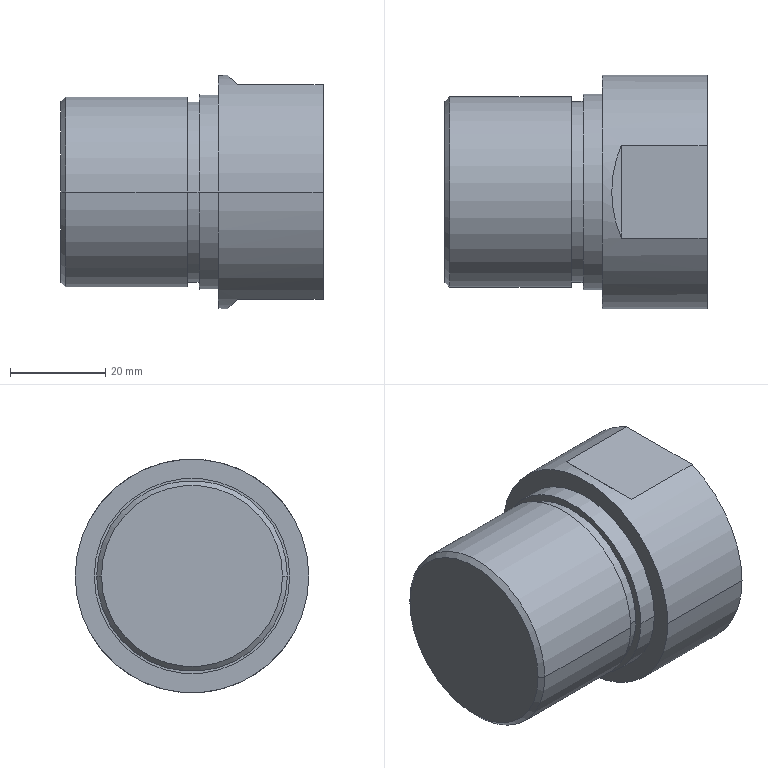Part | SolidWorks | features ICE 5, BaseBody 1, Chamfer 1, HoleWzd 1, MoveFace 1 | 1 solid | 23 faces | box 55 x 49 x 49 mm | volume 69401 mm3 | cylinder 10 | plane 9 | cone 4 | commonest cylinder face diameters 18.5 x2 38 x2 40 x2 41 x2 49 x2
STEP:
#1=CARTESIAN_POINT('',(-2.5,0.,9.25));
#2=VERTEX_POINT('',#1);
#3=CARTESIAN_POINT('',(-2.5,0.,-9.25));
#4=VERTEX_POINT('',#3);
#5=CARTESIAN_POINT('',(-2.5,0.,0.));
#6=DIRECTION('',(1.,0.,0.));
#7=DIRECTION('',(0.,0.,-1.));
#8=AXIS2_PLACEMENT_3D('',#5,#6,#7);
#9=CIRCLE('',#8,9.25);
#10=EDGE_CURVE('',#2,#4,#9,.T.);
#11=ORIENTED_EDGE('',*,*,#10,.F.);
#12=CARTESIAN_POINT('',(42.,0.,9.25));
#13=VERTEX_POINT('',#12);
#14=CARTESIAN_POINT('',(42.,0.,9.25));
#15=DIRECTION('',(1.,0.,0.));
#16=VECTOR('',#15,1000.);
#17=LINE('',#14,#16);
#18=EDGE_CURVE('',#2,#13,#17,.T.);
#19=ORIENTED_EDGE('',*,*,#18,.T.);
#20=CARTESIAN_POINT('',(42.,0.,-9.25));
#21=VERTEX_POINT('',#20);
#22=CARTESIAN_POINT('',(42.,0.,0.));
#23=DIRECTION('',(1.,0.,0.));
#24=DIRECTION('',(0.,0.,-1.));
#25=AXIS2_PLACEMENT_3D('',#22,#23,#24);
#26=CIRCLE('',#25,9.25);
#27=EDGE_CURVE('',#13,#21,#26,.T.);
#28=ORIENTED_EDGE('',*,*,#27,.T.);
#29=CARTESIAN_POINT('',(42.,0.,-9.25));
#30=DIRECTION('',(1.,0.,0.));
#31=VECTOR('',#30,1000.);
#32=LINE('',#29,#31);
#33=EDGE_CURVE('',#4,#21,#32,.T.);
#34=ORIENTED_EDGE('',*,*,#33,.F.);
#35=EDGE_LOOP('',(#11,#19,#28,#34));
#36=FACE_OUTER_BOUND('',#35,.T.);
#37=CARTESIAN_POINT('',(42.,0.,0.));
#38=DIRECTION('',(1.,0.,0.));
#39=DIRECTION('',(0.,0.,-1.));
#40=AXIS2_PLACEMENT_3D('',#37,#38,#39);
#41=CYLINDRICAL_SURFACE('',#40,9.25);
#42=ADVANCED_FACE('',(#36),#41,.F.);
#43=CARTESIAN_POINT('',(-8.058,0.,0.));
#44=VERTEX_POINT('',#43);
#45=CARTESIAN_POINT('',(-2.5,0.,-9.25));
#46=DIRECTION('',(0.515,0.,-0.8572));
#47=VECTOR('',#46,1000.);
#48=LINE('',#45,#47);
#49=EDGE_CURVE('',#44,#4,#48,.T.);
#50=ORIENTED_EDGE('',*,*,#49,.F.);
#51=CARTESIAN_POINT('',(-2.5,0.,9.25));
#52=DIRECTION('',(0.515,0.,0.8572));
#53=VECTOR('',#52,1000.);
#54=LINE('',#51,#53);
#55=EDGE_CURVE('',#44,#2,#54,.T.);
#56=ORIENTED_EDGE('',*,*,#55,.T.);
#57=ORIENTED_EDGE('',*,*,#10,.T.);
#58=EDGE_LOOP('',(#50,#56,#57));
#59=FACE_OUTER_BOUND('',#58,.T.);
#60=CARTESIAN_POINT('',(-2.5,0.,0.));
#61=DIRECTION('',(1.,0.,0.));
#62=DIRECTION('',(0.,0.,-1.));
#63=AXIS2_PLACEMENT_3D('',#60,#61,#62);
#64=CONICAL_SURFACE('',#63,9.25,1.03);
#65=ADVANCED_FACE('',(#59),#64,.F.);
#66=CARTESIAN_POINT('',(42.,24.5,0.));
#67=VERTEX_POINT('',#66);
#68=CARTESIAN_POINT('',(42.,9.695,22.5));
#69=VERTEX_POINT('',#68);
#70=CARTESIAN_POINT('',(42.,0.,0.));
#71=DIRECTION('',(1.,0.,0.));
#72=DIRECTION('',(0.,-1.,0.));
#73=AXIS2_PLACEMENT_3D('',#70,#71,#72);
#74=CIRCLE('',#73,24.5);
#75=EDGE_CURVE('',#67,#69,#74,.T.);
#76=ORIENTED_EDGE('',*,*,#75,.F.);
#77=CARTESIAN_POINT('',(20.,24.5,0.));
#78=VERTEX_POINT('',#77);
#79=CARTESIAN_POINT('',(42.,24.5,0.));
#80=DIRECTION('',(-1.,0.,0.));
#81=VECTOR('',#80,1000.);
#82=LINE('',#79,#81);
#83=EDGE_CURVE('',#67,#78,#82,.T.);
#84=ORIENTED_EDGE('',*,*,#83,.T.);
#85=CARTESIAN_POINT('',(20.,-24.5,0.));
#86=VERTEX_POINT('',#85);
#87=CARTESIAN_POINT('',(20.,0.,0.));
#88=DIRECTION('',(1.,0.,0.));
#89=DIRECTION('',(0.,-1.,0.));
#90=AXIS2_PLACEMENT_3D('',#87,#88,#89);
#91=CIRCLE('',#90,24.5);
#92=EDGE_CURVE('',#78,#86,#91,.T.);
#93=ORIENTED_EDGE('',*,*,#92,.T.);
#94=CARTESIAN_POINT('',(42.,-24.5,0.));
#95=VERTEX_POINT('',#94);
#96=CARTESIAN_POINT('',(42.,-24.5,0.));
#97=DIRECTION('',(-1.,0.,0.));
#98=VECTOR('',#97,1000.);
#99=LINE('',#96,#98);
#100=EDGE_CURVE('',#95,#86,#99,.T.);
#101=ORIENTED_EDGE('',*,*,#100,.F.);
#102=CARTESIAN_POINT('',(42.,-9.695,22.5));
#103=VERTEX_POINT('',#102);
#104=CARTESIAN_POINT('',(42.,0.,0.));
#105=DIRECTION('',(1.,0.,0.));
#106=DIRECTION('',(0.,-1.,0.));
#107=AXIS2_PLACEMENT_3D('',#104,#105,#106);
#108=CIRCLE('',#107,24.5);
#109=EDGE_CURVE('',#103,#95,#108,.T.);
#110=ORIENTED_EDGE('',*,*,#109,.F.);
#111=CARTESIAN_POINT('',(24.,-9.695,22.5));
#112=VERTEX_POINT('',#111);
#113=CARTESIAN_POINT('',(42.,-9.695,22.5));
#114=DIRECTION('',(-1.,0.,0.));
#115=VECTOR('',#114,1000.);
#116=LINE('',#113,#115);
#117=EDGE_CURVE('',#103,#112,#116,.T.);
#118=ORIENTED_EDGE('',*,*,#117,.T.);
#119=CARTESIAN_POINT('',(24.,9.695,22.5));
#120=VERTEX_POINT('',#119);
#121=CARTESIAN_POINT('',(24.,-9.695,22.5));
#122=CARTESIAN_POINT('',(21.295,-3.418,25.205));
#123=CARTESIAN_POINT('',(21.295,3.418,25.205));
#124=CARTESIAN_POINT('',(24.,9.695,22.5));
#125=(BOUNDED_CURVE()B_SPLINE_CURVE(3,(#121,#122,#123,#124),.UNSPECIFIED.,.F.,.F.)B_SPLINE_CURVE_WITH_KNOTS((4,4),(5.876,6.69),.UNSPECIFIED.)CURVE()GEOMETRIC_REPRESENTATION_ITEM()RATIONAL_B_SPLINE_CURVE((1.,0.9456,0.9456,1.))REPRESENTATION_ITEM(''));
#126=EDGE_CURVE('',#112,#120,#125,.T.);
#127=ORIENTED_EDGE('',*,*,#126,.T.);
#128=CARTESIAN_POINT('',(42.,9.695,22.5));
#129=DIRECTION('',(1.,0.,0.));
#130=VECTOR('',#129,1000.);
#131=LINE('',#128,#130);
#132=EDGE_CURVE('',#120,#69,#131,.T.);
#133=ORIENTED_EDGE('',*,*,#132,.T.);
#134=EDGE_LOOP('',(#76,#84,#93,#101,#110,#118,#127,#133));
#135=FACE_OUTER_BOUND('',#134,.T.);
#136=CARTESIAN_POINT('',(42.,0.,0.));
#137=DIRECTION('',(-1.,0.,0.));
#138=DIRECTION('',(0.,-1.,0.));
#139=AXIS2_PLACEMENT_3D('',#136,#137,#138);
#140=CYLINDRICAL_SURFACE('',#139,24.5);
#141=ADVANCED_FACE('',(#135),#140,.T.);
#142=CARTESIAN_POINT('',(16.,20.5,0.));
#143=VERTEX_POINT('',#142);
#144=CARTESIAN_POINT('',(16.,-20.5,0.));
#145=VERTEX_POINT('',#144);
#146=CARTESIAN_POINT('',(16.,0.,0.));
#147=DIRECTION('',(1.,0.,0.));
#148=DIRECTION('',(0.,1.,0.));
#149=AXIS2_PLACEMENT_3D('',#146,#147,#148);
#150=CIRCLE('',#149,20.5);
#151=EDGE_CURVE('',#143,#145,#150,.T.);
#152=ORIENTED_EDGE('',*,*,#151,.T.);
#153=CARTESIAN_POINT('',(20.,-20.5,0.));
#154=VERTEX_POINT('',#153);
#155=CARTESIAN_POINT('',(16.,-20.5,0.));
#156=DIRECTION('',(1.,0.,0.));
#157=VECTOR('',#156,1000.);
#158=LINE('',#155,#157);
#159=EDGE_CURVE('',#145,#154,#158,.T.);
#160=ORIENTED_EDGE('',*,*,#159,.T.);
#161=CARTESIAN_POINT('',(20.,20.5,0.));
#162=VERTEX_POINT('',#161);
#163=CARTESIAN_POINT('',(20.,0.,0.));
#164=DIRECTION('',(1.,0.,0.));
#165=DIRECTION('',(0.,1.,0.));
#166=AXIS2_PLACEMENT_3D('',#163,#164,#165);
#167=CIRCLE('',#166,20.5);
#168=EDGE_CURVE('',#162,#154,#167,.T.);
#169=ORIENTED_EDGE('',*,*,#168,.F.);
#170=CARTESIAN_POINT('',(16.,20.5,0.));
#171=DIRECTION('',(1.,0.,0.));
#172=VECTOR('',#171,1000.);
#173=LINE('',#170,#172);
#174=EDGE_CURVE('',#143,#162,#173,.T.);
#175=ORIENTED_EDGE('',*,*,#174,.F.);
#176=EDGE_LOOP('',(#152,#160,#169,#175));
#177=FACE_OUTER_BOUND('',#176,.T.);
#178=CARTESIAN_POINT('',(16.,0.,0.));
#179=DIRECTION('',(1.,0.,0.));
#180=DIRECTION('',(0.,1.,0.));
#181=AXIS2_PLACEMENT_3D('',#178,#179,#180);
#182=CYLINDRICAL_SURFACE('',#181,20.5);
#183=ADVANCED_FACE('',(#177),#182,.T.);
#184=CARTESIAN_POINT('',(13.5,19.,0.));
#185=VERTEX_POINT('',#184);
#186=CARTESIAN_POINT('',(13.5,-19.,0.));
#187=VERTEX_POINT('',#186);
#188=CARTESIAN_POINT('',(13.5,0.,0.));
#189=DIRECTION('',(1.,0.,0.));
#190=DIRECTION('',(0.,1.,0.));
#191=AXIS2_PLACEMENT_3D('',#188,#189,#190);
#192=CIRCLE('',#191,19.);
#193=EDGE_CURVE('',#185,#187,#192,.T.);
#194=ORIENTED_EDGE('',*,*,#193,.T.);
#195=CARTESIAN_POINT('',(16.,-19.,0.));
#196=VERTEX_POINT('',#195);
#197=CARTESIAN_POINT('',(13.5,-19.,0.));
#198=DIRECTION('',(1.,0.,0.));
#199=VECTOR('',#198,1000.);
#200=LINE('',#197,#199);
#201=EDGE_CURVE('',#187,#196,#200,.T.);
#202=ORIENTED_EDGE('',*,*,#201,.T.);
#203=CARTESIAN_POINT('',(16.,19.,0.));
#204=VERTEX_POINT('',#203);
#205=CARTESIAN_POINT('',(16.,0.,0.));
#206=DIRECTION('',(1.,0.,0.));
#207=DIRECTION('',(0.,1.,0.));
#208=AXIS2_PLACEMENT_3D('',#205,#206,#207);
#209=CIRCLE('',#208,19.);
#210=EDGE_CURVE('',#204,#196,#209,.T.);
#211=ORIENTED_EDGE('',*,*,#210,.F.);
#212=CARTESIAN_POINT('',(13.5,19.,0.));
#213=DIRECTION('',(1.,0.,0.));
#214=VECTOR('',#213,1000.);
#215=LINE('',#212,#214);
#216=EDGE_CURVE('',#185,#204,#215,.T.);
#217=ORIENTED_EDGE('',*,*,#216,.F.);
#218=EDGE_LOOP('',(#194,#202,#211,#217));
#219=FACE_OUTER_BOUND('',#218,.T.);
#220=CARTESIAN_POINT('',(13.5,0.,0.));
#221=DIRECTION('',(1.,0.,0.));
#222=DIRECTION('',(0.,1.,0.));
#223=AXIS2_PLACEMENT_3D('',#220,#221,#222);
#224=CYLINDRICAL_SURFACE('',#223,19.);
#225=ADVANCED_FACE('',(#219),#224,.T.);
#226=CARTESIAN_POINT('',(-12.,20.,0.));
#227=VERTEX_POINT('',#226);
#228=CARTESIAN_POINT('',(-12.,-20.,0.));
#229=VERTEX_POINT('',#228);
#230=CARTESIAN_POINT('',(-12.,0.,0.));
#231=DIRECTION('',(1.,0.,0.));
#232=DIRECTION('',(0.,1.,0.));
#233=AXIS2_PLACEMENT_3D('',#230,#231,#232);
#234=CIRCLE('',#233,20.);
#235=EDGE_CURVE('',#227,#229,#234,.T.);
#236=ORIENTED_EDGE('',*,*,#235,.T.);
#237=CARTESIAN_POINT('',(13.5,-20.,0.));
#238=VERTEX_POINT('',#237);
#239=CARTESIAN_POINT('',(9.5,-20.,0.));
#240=DIRECTION('',(1.,0.,0.));
#241=VECTOR('',#240,1000.);
#242=LINE('',#239,#241);
#243=EDGE_CURVE('',#229,#238,#242,.T.);
#244=ORIENTED_EDGE('',*,*,#243,.T.);
#245=CARTESIAN_POINT('',(13.5,20.,0.));
#246=VERTEX_POINT('',#245);
#247=CARTESIAN_POINT('',(13.5,0.,0.));
#248=DIRECTION('',(-1.,0.,0.));
#249=DIRECTION('',(0.,1.,0.));
#250=AXIS2_PLACEMENT_3D('',#247,#248,#249);
#251=CIRCLE('',#250,20.);
#252=EDGE_CURVE('',#238,#246,#251,.T.);
#253=ORIENTED_EDGE('',*,*,#252,.T.);
#254=CARTESIAN_POINT('',(9.5,20.,0.));
#255=DIRECTION('',(1.,0.,0.));
#256=VECTOR('',#255,1000.);
#257=LINE('',#254,#256);
#258=EDGE_CURVE('',#227,#246,#257,.T.);
#259=ORIENTED_EDGE('',*,*,#258,.F.);
#260=EDGE_LOOP('',(#236,#244,#253,#259));
#261=FACE_OUTER_BOUND('',#260,.T.);
#262=CARTESIAN_POINT('',(9.5,0.,0.));
#263=DIRECTION('',(1.,0.,0.));
#264=DIRECTION('',(0.,1.,0.));
#265=AXIS2_PLACEMENT_3D('',#262,#263,#264);
#266=CYLINDRICAL_SURFACE('',#265,20.);
#267=ADVANCED_FACE('',(#261),#266,.T.);
#268=CARTESIAN_POINT('',(-13.,19.,0.));
#269=VERTEX_POINT('',#268);
#270=CARTESIAN_POINT('',(-13.,-19.,0.));
#271=VERTEX_POINT('',#270);
#272=CARTESIAN_POINT('',(-13.,0.,0.));
#273=DIRECTION('',(1.,0.,0.));
#274=DIRECTION('',(0.,1.,0.));
#275=AXIS2_PLACEMENT_3D('',#272,#273,#274);
#276=CIRCLE('',#275,19.);
#277=EDGE_CURVE('',#269,#271,#276,.T.);
#278=ORIENTED_EDGE('',*,*,#277,.T.);
#279=CARTESIAN_POINT('',(-12.,-20.,0.));
#280=DIRECTION('',(0.7071,-0.7071,0.));
#281=VECTOR('',#280,1000.);
#282=LINE('',#279,#281);
#283=EDGE_CURVE('',#271,#229,#282,.T.);
#284=ORIENTED_EDGE('',*,*,#283,.T.);
#285=ORIENTED_EDGE('',*,*,#235,.F.);
#286=CARTESIAN_POINT('',(-12.,20.,0.));
#287=DIRECTION('',(0.7071,0.7071,0.));
#288=VECTOR('',#287,1000.);
#289=LINE('',#286,#288);
#290=EDGE_CURVE('',#269,#227,#289,.T.);
#291=ORIENTED_EDGE('',*,*,#290,.F.);
#292=EDGE_LOOP('',(#278,#284,#285,#291));
#293=FACE_OUTER_BOUND('',#292,.T.);
#294=CARTESIAN_POINT('',(-12.,0.,0.));
#295=DIRECTION('',(1.,0.,0.));
#296=DIRECTION('',(0.,1.,0.));
#297=AXIS2_PLACEMENT_3D('',#294,#295,#296);
#298=CONICAL_SURFACE('',#297,20.,0.7854);
#299=ADVANCED_FACE('',(#293),#298,.T.);
#300=CARTESIAN_POINT('',(42.,0.,0.));
#301=DIRECTION('',(1.,0.,0.));
#302=DIRECTION('',(0.,0.,-1.));
#303=AXIS2_PLACEMENT_3D('',#300,#301,#302);
#304=CIRCLE('',#303,9.25);
#305=EDGE_CURVE('',#21,#13,#304,.T.);
#306=ORIENTED_EDGE('',*,*,#305,.F.);
#307=ORIENTED_EDGE('',*,*,#27,.F.);
#308=EDGE_LOOP('',(#306,#307));
#309=FACE_BOUND('',#308,.T.);
#310=CARTESIAN_POINT('',(42.,21.5,22.5));
#311=DIRECTION('',(0.,-1.,0.));
#312=VECTOR('',#311,1000.);
#313=LINE('',#310,#312);
#314=EDGE_CURVE('',#69,#103,#313,.T.);
#315=ORIENTED_EDGE('',*,*,#314,.T.);
#316=ORIENTED_EDGE('',*,*,#109,.T.);
#317=CARTESIAN_POINT('',(42.,-9.695,-22.5));
#318=VERTEX_POINT('',#317);
#319=CARTESIAN_POINT('',(42.,0.,0.));
#320=DIRECTION('',(1.,0.,0.));
#321=DIRECTION('',(0.,-1.,0.));
#322=AXIS2_PLACEMENT_3D('',#319,#320,#321);
#323=CIRCLE('',#322,24.5);
#324=EDGE_CURVE('',#95,#318,#323,.T.);
#325=ORIENTED_EDGE('',*,*,#324,.T.);
#326=CARTESIAN_POINT('',(42.,9.695,-22.5));
#327=VERTEX_POINT('',#326);
#328=CARTESIAN_POINT('',(42.,21.5,-22.5));
#329=DIRECTION('',(0.,1.,0.));
#330=VECTOR('',#329,1000.);
#331=LINE('',#328,#330);
#332=EDGE_CURVE('',#318,#327,#331,.T.);
#333=ORIENTED_EDGE('',*,*,#332,.T.);
#334=CARTESIAN_POINT('',(42.,0.,0.));
#335=DIRECTION('',(1.,0.,0.));
#336=DIRECTION('',(0.,-1.,0.));
#337=AXIS2_PLACEMENT_3D('',#334,#335,#336);
#338=CIRCLE('',#337,24.5);
#339=EDGE_CURVE('',#327,#67,#338,.T.);
#340=ORIENTED_EDGE('',*,*,#339,.T.);
#341=ORIENTED_EDGE('',*,*,#75,.T.);
#342=EDGE_LOOP('',(#315,#316,#325,#333,#340,#341));
#343=FACE_OUTER_BOUND('',#342,.T.);
#344=CARTESIAN_POINT('',(42.,21.5,0.));
#345=DIRECTION('',(1.,0.,0.));
#346=DIRECTION('',(0.,0.,-1.));
#347=AXIS2_PLACEMENT_3D('',#344,#345,#346);
#348=PLANE('',#347);
#349=ADVANCED_FACE('',(#309,#343),#348,.T.);
#350=ORIENTED_EDGE('',*,*,#83,.F.);
#351=ORIENTED_EDGE('',*,*,#339,.F.);
#352=CARTESIAN_POINT('',(24.,9.695,-22.5));
#353=VERTEX_POINT('',#352);
#354=CARTESIAN_POINT('',(42.,9.695,-22.5));
#355=DIRECTION('',(-1.,0.,0.));
#356=VECTOR('',#355,1000.);
#357=LINE('',#354,#356);
#358=EDGE_CURVE('',#327,#353,#357,.T.);
#359=ORIENTED_EDGE('',*,*,#358,.T.);
#360=CARTESIAN_POINT('',(24.,-9.695,-22.5));
#361=VERTEX_POINT('',#360);
#362=CARTESIAN_POINT('',(24.,9.695,-22.5));
#363=CARTESIAN_POINT('',(21.295,3.418,-25.205));
#364=CARTESIAN_POINT('',(21.295,-3.418,-25.205));
#365=CARTESIAN_POINT('',(24.,-9.695,-22.5));
#366=(BOUNDED_CURVE()B_SPLINE_CURVE(3,(#362,#363,#364,#365),.UNSPECIFIED.,.F.,.F.)B_SPLINE_CURVE_WITH_KNOTS((4,4),(5.876,6.69),.UNSPECIFIED.)CURVE()GEOMETRIC_REPRESENTATION_ITEM()RATIONAL_B_SPLINE_CURVE((1.,0.9456,0.9456,1.))REPRESENTATION_ITEM(''));
#367=EDGE_CURVE('',#353,#361,#366,.T.);
#368=ORIENTED_EDGE('',*,*,#367,.T.);
#369=CARTESIAN_POINT('',(42.,-9.695,-22.5));
#370=DIRECTION('',(1.,0.,0.));
#371=VECTOR('',#370,1000.);
#372=LINE('',#369,#371);
#373=EDGE_CURVE('',#361,#318,#372,.T.);
#374=ORIENTED_EDGE('',*,*,#373,.T.);
#375=ORIENTED_EDGE('',*,*,#324,.F.);
#376=ORIENTED_EDGE('',*,*,#100,.T.);
#377=CARTESIAN_POINT('',(20.,0.,0.));
#378=DIRECTION('',(1.,0.,0.));
#379=DIRECTION('',(0.,-1.,0.));
#380=AXIS2_PLACEMENT_3D('',#377,#378,#379);
#381=CIRCLE('',#380,24.5);
#382=EDGE_CURVE('',#86,#78,#381,.T.);
#383=ORIENTED_EDGE('',*,*,#382,.T.);
#384=EDGE_LOOP('',(#350,#351,#359,#368,#374,#375,#376,#383));
#385=FACE_OUTER_BOUND('',#384,.T.);
#386=CARTESIAN_POINT('',(42.,0.,0.));
#387=DIRECTION('',(-1.,0.,0.));
#388=DIRECTION('',(0.,-1.,0.));
#389=AXIS2_PLACEMENT_3D('',#386,#387,#388);
#390=CYLINDRICAL_SURFACE('',#389,24.5);
#391=ADVANCED_FACE('',(#385),#390,.T.);
#392=ORIENTED_EDGE('',*,*,#314,.F.);
#393=ORIENTED_EDGE('',*,*,#132,.F.);
#394=CARTESIAN_POINT('',(24.,0.,22.5));
#395=DIRECTION('',(0.,1.,0.));
#396=VECTOR('',#395,1000.);
#397=LINE('',#394,#396);
#398=EDGE_CURVE('',#112,#120,#397,.T.);
#399=ORIENTED_EDGE('',*,*,#398,.F.);
#400=ORIENTED_EDGE('',*,*,#117,.F.);
#401=EDGE_LOOP('',(#392,#393,#399,#400));
#402=FACE_OUTER_BOUND('',#401,.T.);
#403=CARTESIAN_POINT('',(42.,0.,22.5));
#404=DIRECTION('',(0.,0.,-1.));
#405=DIRECTION('',(-1.,0.,0.));
#406=AXIS2_PLACEMENT_3D('',#403,#404,#405);
#407=PLANE('',#406);
#408=ADVANCED_FACE('',(#402),#407,.F.);
#409=ORIENTED_EDGE('',*,*,#332,.F.);
#410=ORIENTED_EDGE('',*,*,#373,.F.);
#411=CARTESIAN_POINT('',(24.,0.,-22.5));
#412=DIRECTION('',(0.,-1.,0.));
#413=VECTOR('',#412,1000.);
#414=LINE('',#411,#413);
#415=EDGE_CURVE('',#353,#361,#414,.T.);
#416=ORIENTED_EDGE('',*,*,#415,.F.);
#417=ORIENTED_EDGE('',*,*,#358,.F.);
#418=EDGE_LOOP('',(#409,#410,#416,#417));
#419=FACE_OUTER_BOUND('',#418,.T.);
#420=CARTESIAN_POINT('',(42.,0.,-22.5));
#421=DIRECTION('',(0.,0.,1.));
#422=DIRECTION('',(1.,0.,0.));
#423=AXIS2_PLACEMENT_3D('',#420,#421,#422);
#424=PLANE('',#423);
#425=ADVANCED_FACE('',(#419),#424,.F.);
#426=ORIENTED_EDGE('',*,*,#168,.T.);
#427=CARTESIAN_POINT('',(20.,0.,0.));
#428=DIRECTION('',(1.,0.,0.));
#429=DIRECTION('',(0.,1.,0.));
#430=AXIS2_PLACEMENT_3D('',#427,#428,#429);
#431=CIRCLE('',#430,20.5);
#432=EDGE_CURVE('',#154,#162,#431,.T.);
#433=ORIENTED_EDGE('',*,*,#432,.T.);
#434=EDGE_LOOP('',(#426,#433));
#435=FACE_BOUND('',#434,.T.);
#436=ORIENTED_EDGE('',*,*,#382,.F.);
#437=ORIENTED_EDGE('',*,*,#92,.F.);
#438=EDGE_LOOP('',(#436,#437));
#439=FACE_OUTER_BOUND('',#438,.T.);
#440=CARTESIAN_POINT('',(20.,22.5,0.));
#441=DIRECTION('',(-1.,0.,0.));
#442=DIRECTION('',(0.,-1.,0.));
#443=AXIS2_PLACEMENT_3D('',#440,#441,#442);
#444=PLANE('',#443);
#445=ADVANCED_FACE('',(#435,#439),#444,.T.);
#446=ORIENTED_EDGE('',*,*,#415,.T.);
#447=ORIENTED_EDGE('',*,*,#367,.F.);
#448=EDGE_LOOP('',(#446,#447));
#449=FACE_OUTER_BOUND('',#448,.T.);
#450=CARTESIAN_POINT('',(24.,0.,-22.5));
#451=DIRECTION('',(0.7071,0.,-0.7071));
#452=DIRECTION('',(-0.7071,0.,-0.7071));
#453=AXIS2_PLACEMENT_3D('',#450,#451,#452);
#454=PLANE('',#453);
#455=ADVANCED_FACE('',(#449),#454,.T.);
#456=ORIENTED_EDGE('',*,*,#398,.T.);
#457=ORIENTED_EDGE('',*,*,#126,.F.);
#458=EDGE_LOOP('',(#456,#457));
#459=FACE_OUTER_BOUND('',#458,.T.);
#460=CARTESIAN_POINT('',(24.,0.,22.5));
#461=DIRECTION('',(0.7071,0.,0.7071));
#462=DIRECTION('',(0.7071,0.,-0.7071));
#463=AXIS2_PLACEMENT_3D('',#460,#461,#462);
#464=PLANE('',#463);
#465=ADVANCED_FACE('',(#459),#464,.T.);
#466=ORIENTED_EDGE('',*,*,#159,.F.);
#467=CARTESIAN_POINT('',(16.,0.,0.));
#468=DIRECTION('',(1.,0.,0.));
#469=DIRECTION('',(0.,1.,0.));
#470=AXIS2_PLACEMENT_3D('',#467,#468,#469);
#471=CIRCLE('',#470,20.5);
#472=EDGE_CURVE('',#145,#143,#471,.T.);
#473=ORIENTED_EDGE('',*,*,#472,.T.);
#474=ORIENTED_EDGE('',*,*,#174,.T.);
#475=ORIENTED_EDGE('',*,*,#432,.F.);
#476=EDGE_LOOP('',(#466,#473,#474,#475));
#477=FACE_OUTER_BOUND('',#476,.T.);
#478=CARTESIAN_POINT('',(16.,0.,0.));
#479=DIRECTION('',(1.,0.,0.));
#480=DIRECTION('',(0.,1.,0.));
#481=AXIS2_PLACEMENT_3D('',#478,#479,#480);
#482=CYLINDRICAL_SURFACE('',#481,20.5);
#483=ADVANCED_FACE('',(#477),#482,.T.);
#484=ORIENTED_EDGE('',*,*,#210,.T.);
#485=CARTESIAN_POINT('',(16.,0.,0.));
#486=DIRECTION('',(1.,0.,0.));
#487=DIRECTION('',(0.,1.,0.));
#488=AXIS2_PLACEMENT_3D('',#485,#486,#487);
#489=CIRCLE('',#488,19.);
#490=EDGE_CURVE('',#196,#204,#489,.T.);
#491=ORIENTED_EDGE('',*,*,#490,.T.);
#492=EDGE_LOOP('',(#484,#491));
#493=FACE_BOUND('',#492,.T.);
#494=ORIENTED_EDGE('',*,*,#151,.F.);
#495=ORIENTED_EDGE('',*,*,#472,.F.);
#496=EDGE_LOOP('',(#494,#495));
#497=FACE_OUTER_BOUND('',#496,.T.);
#498=CARTESIAN_POINT('',(16.,0.,0.));
#499=DIRECTION('',(-1.,0.,0.));
#500=DIRECTION('',(0.,-1.,0.));
#501=AXIS2_PLACEMENT_3D('',#498,#499,#500);
#502=PLANE('',#501);
#503=ADVANCED_FACE('',(#493,#497),#502,.T.);
#504=ORIENTED_EDGE('',*,*,#201,.F.);
#505=CARTESIAN_POINT('',(13.5,0.,0.));
#506=DIRECTION('',(1.,0.,0.));
#507=DIRECTION('',(0.,1.,0.));
#508=AXIS2_PLACEMENT_3D('',#505,#506,#507);
#509=CIRCLE('',#508,19.);
#510=EDGE_CURVE('',#187,#185,#509,.T.);
#511=ORIENTED_EDGE('',*,*,#510,.T.);
#512=ORIENTED_EDGE('',*,*,#216,.T.);
#513=ORIENTED_EDGE('',*,*,#490,.F.);
#514=EDGE_LOOP('',(#504,#511,#512,#513));
#515=FACE_OUTER_BOUND('',#514,.T.);
#516=CARTESIAN_POINT('',(13.5,0.,0.));
#517=DIRECTION('',(1.,0.,0.));
#518=DIRECTION('',(0.,1.,0.));
#519=AXIS2_PLACEMENT_3D('',#516,#517,#518);
#520=CYLINDRICAL_SURFACE('',#519,19.);
#521=ADVANCED_FACE('',(#515),#520,.T.);
#522=ORIENTED_EDGE('',*,*,#193,.F.);
#523=ORIENTED_EDGE('',*,*,#510,.F.);
#524=EDGE_LOOP('',(#522,#523));
#525=FACE_BOUND('',#524,.T.);
#526=CARTESIAN_POINT('',(13.5,0.,0.));
#527=DIRECTION('',(-1.,0.,0.));
#528=DIRECTION('',(0.,1.,0.));
#529=AXIS2_PLACEMENT_3D('',#526,#527,#528);
#530=CIRCLE('',#529,20.);
#531=EDGE_CURVE('',#246,#238,#530,.T.);
#532=ORIENTED_EDGE('',*,*,#531,.F.);
#533=ORIENTED_EDGE('',*,*,#252,.F.);
#534=EDGE_LOOP('',(#532,#533));
#535=FACE_OUTER_BOUND('',#534,.T.);
#536=CARTESIAN_POINT('',(13.5,0.,0.));
#537=DIRECTION('',(-1.,0.,0.));
#538=DIRECTION('',(0.,-1.,0.));
#539=AXIS2_PLACEMENT_3D('',#536,#537,#538);
#540=PLANE('',#539);
#541=ADVANCED_FACE('',(#525,#535),#540,.F.);
#542=ORIENTED_EDGE('',*,*,#243,.F.);
#543=CARTESIAN_POINT('',(-12.,0.,0.));
#544=DIRECTION('',(1.,0.,0.));
#545=DIRECTION('',(0.,1.,0.));
#546=AXIS2_PLACEMENT_3D('',#543,#544,#545);
#547=CIRCLE('',#546,20.);
#548=EDGE_CURVE('',#229,#227,#547,.T.);
#549=ORIENTED_EDGE('',*,*,#548,.T.);
#550=ORIENTED_EDGE('',*,*,#258,.T.);
#551=ORIENTED_EDGE('',*,*,#531,.T.);
#552=EDGE_LOOP('',(#542,#549,#550,#551));
#553=FACE_OUTER_BOUND('',#552,.T.);
#554=CARTESIAN_POINT('',(9.5,0.,0.));
#555=DIRECTION('',(1.,0.,0.));
#556=DIRECTION('',(0.,1.,0.));
#557=AXIS2_PLACEMENT_3D('',#554,#555,#556);
#558=CYLINDRICAL_SURFACE('',#557,20.);
#559=ADVANCED_FACE('',(#553),#558,.T.);
#560=ORIENTED_EDGE('',*,*,#283,.F.);
#561=CARTESIAN_POINT('',(-13.,0.,0.));
#562=DIRECTION('',(1.,0.,0.));
#563=DIRECTION('',(0.,1.,0.));
#564=AXIS2_PLACEMENT_3D('',#561,#562,#563);
#565=CIRCLE('',#564,19.);
#566=EDGE_CURVE('',#271,#269,#565,.T.);
#567=ORIENTED_EDGE('',*,*,#566,.T.);
#568=ORIENTED_EDGE('',*,*,#290,.T.);
#569=ORIENTED_EDGE('',*,*,#548,.F.);
#570=EDGE_LOOP('',(#560,#567,#568,#569));
#571=FACE_OUTER_BOUND('',#570,.T.);
#572=CARTESIAN_POINT('',(-12.,0.,0.));
#573=DIRECTION('',(1.,0.,0.));
#574=DIRECTION('',(0.,1.,0.));
#575=AXIS2_PLACEMENT_3D('',#572,#573,#574);
#576=CONICAL_SURFACE('',#575,20.,0.7854);
#577=ADVANCED_FACE('',(#571),#576,.T.);
#578=ORIENTED_EDGE('',*,*,#277,.F.);
#579=ORIENTED_EDGE('',*,*,#566,.F.);
#580=EDGE_LOOP('',(#578,#579));
#581=FACE_OUTER_BOUND('',#580,.T.);
#582=CARTESIAN_POINT('',(-13.,0.,0.));
#583=DIRECTION('',(1.,0.,0.));
#584=DIRECTION('',(0.,1.,0.));
#585=AXIS2_PLACEMENT_3D('',#582,#583,#584);
#586=PLANE('',#585);
#587=ADVANCED_FACE('',(#581),#586,.F.);
#588=ORIENTED_EDGE('',*,*,#55,.F.);
#589=ORIENTED_EDGE('',*,*,#49,.T.);
#590=CARTESIAN_POINT('',(-2.5,0.,0.));
#591=DIRECTION('',(1.,0.,0.));
#592=DIRECTION('',(0.,0.,-1.));
#593=AXIS2_PLACEMENT_3D('',#590,#591,#592);
#594=CIRCLE('',#593,9.25);
#595=EDGE_CURVE('',#4,#2,#594,.T.);
#596=ORIENTED_EDGE('',*,*,#595,.T.);
#597=EDGE_LOOP('',(#588,#589,#596));
#598=FACE_OUTER_BOUND('',#597,.T.);
#599=CARTESIAN_POINT('',(-2.5,0.,0.));
#600=DIRECTION('',(1.,0.,0.));
#601=DIRECTION('',(0.,0.,-1.));
#602=AXIS2_PLACEMENT_3D('',#599,#600,#601);
#603=CONICAL_SURFACE('',#602,9.25,1.03);
#604=ADVANCED_FACE('',(#598),#603,.F.);
#605=ORIENTED_EDGE('',*,*,#18,.F.);
#606=ORIENTED_EDGE('',*,*,#595,.F.);
#607=ORIENTED_EDGE('',*,*,#33,.T.);
#608=ORIENTED_EDGE('',*,*,#305,.T.);
#609=EDGE_LOOP('',(#605,#606,#607,#608));
#610=FACE_OUTER_BOUND('',#609,.T.);
#611=CARTESIAN_POINT('',(42.,0.,0.));
#612=DIRECTION('',(1.,0.,0.));
#613=DIRECTION('',(0.,0.,-1.));
#614=AXIS2_PLACEMENT_3D('',#611,#612,#613);
#615=CYLINDRICAL_SURFACE('',#614,9.25);
#616=ADVANCED_FACE('',(#610),#615,.F.);
#617=CLOSED_SHELL('',(#42,#65,#141,#183,#225,#267,#299,#349,#391,#408,#425,#445,#455,#465,#483,#503,#521,#541,#559,#577,#587,#604,#616));
#618=MANIFOLD_SOLID_BREP('',#617);
#619=CARTESIAN_POINT('',(0.,0.,0.));
#620=DIRECTION('',(0.,0.,1.));
#621=DIRECTION('',(1.,0.,0.));
#622=AXIS2_PLACEMENT_3D('',#619,#620,#621);
#623=(LENGTH_UNIT()NAMED_UNIT(*)SI_UNIT(.MILLI.,.METRE.));
#624=UNCERTAINTY_MEASURE_WITH_UNIT(LENGTH_MEASURE(0.00001),#623,'','');
#625=(NAMED_UNIT(*)PLANE_ANGLE_UNIT()SI_UNIT($,.RADIAN.));
#626=(NAMED_UNIT(*)SI_UNIT($,.STERADIAN.)SOLID_ANGLE_UNIT());
#627=(GEOMETRIC_REPRESENTATION_CONTEXT(3)GLOBAL_UNCERTAINTY_ASSIGNED_CONTEXT((#624))GLOBAL_UNIT_ASSIGNED_CONTEXT((#623,#625,#626))REPRESENTATION_CONTEXT('',''));
#628=ADVANCED_BREP_SHAPE_REPRESENTATION('',(#618,#622),#627);